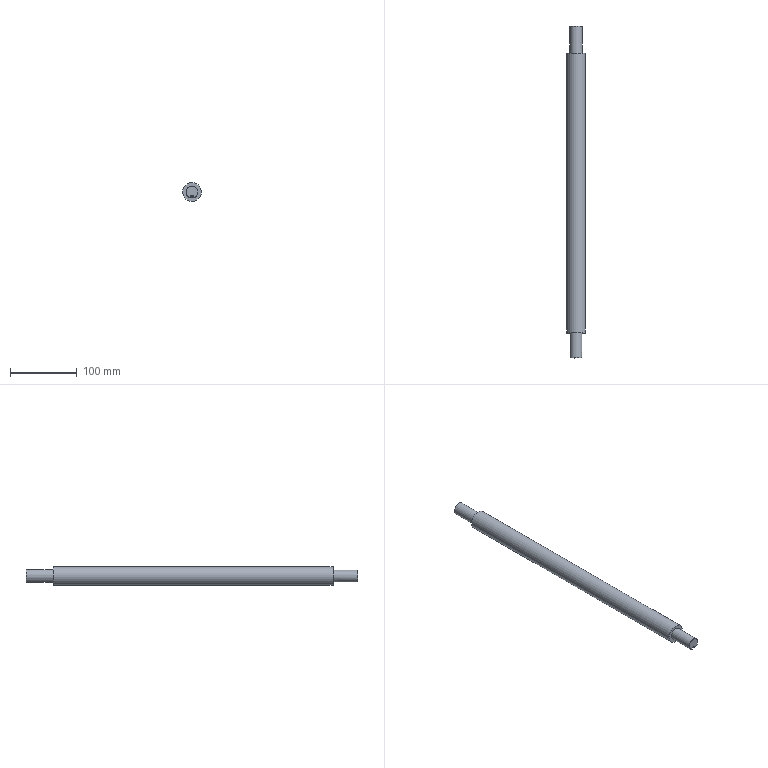Part | STEP file | SN10_002_009-03_EIXO | 1 solid | 15 faces | box 28 x 498.3 x 28 mm | volume 278975 mm3 | plane 8 | cylinder 5 | cone 2 | commonest cylinder face diameters 5 x2 18 x1 19.05 x1 28 x1
STEP:
#1=CARTESIAN_POINT('',(0.,0.,0.));
#2=DIRECTION('',(0.,0.,1.));
#3=DIRECTION('',(1.,0.,0.));
#4=AXIS2_PLACEMENT_3D('',#1,#2,#3);
#5=CARTESIAN_POINT('',(993.288,42.3,12.286));
#6=VERTEX_POINT('',#5);
#7=CARTESIAN_POINT('',(1000.,42.3,0.));
#8=DIRECTION('',(0.,-1.,0.));
#9=DIRECTION('',(1.,0.,0.));
#10=AXIS2_PLACEMENT_3D('',#7,#8,#9);
#11=CIRCLE('',#10,14.);
#12=CARTESIAN_POINT('',(1000.,-165.85,0.));
#13=DIRECTION('',(0.,-1.,0.));
#14=DIRECTION('',(-0.4794,0.,0.8776));
#15=AXIS2_PLACEMENT_3D('',#12,#13,#14);
#16=CYLINDRICAL_SURFACE('',#15,14.);
#17=CARTESIAN_POINT('',(-2.071,-208.15));
#18=DIRECTION('',(1.,0.));
#19=VECTOR('',#18,1.);
#20=LINE('',#17,#19);
#21=(GEOMETRIC_REPRESENTATION_CONTEXT(2)PARAMETRIC_REPRESENTATION_CONTEXT()REPRESENTATION_CONTEXT('',''));
#22=DEFINITIONAL_REPRESENTATION('',(#20),#21);
#23=PCURVE('',#16,#22);
#24=CARTESIAN_POINT('',(1000.,42.3,14.));
#25=DIRECTION('',(0.,-1.,0.));
#26=DIRECTION('',(0.,0.,-1.));
#27=AXIS2_PLACEMENT_3D('',#24,#25,#26);
#28=PLANE('',#27);
#29=CARTESIAN_POINT('',(14.,0.));
#30=DIRECTION('',(0.,1.));
#31=AXIS2_PLACEMENT_2D('',#29,#30);
#32=CIRCLE('',#31,14.);
#33=(GEOMETRIC_REPRESENTATION_CONTEXT(2)PARAMETRIC_REPRESENTATION_CONTEXT()REPRESENTATION_CONTEXT('',''));
#34=DEFINITIONAL_REPRESENTATION('',(#32),#33);
#35=PCURVE('',#28,#34);
#36=SURFACE_CURVE('',#11,(#23,#35),.PCURVE_S1.);
#37=EDGE_CURVE('',#6,#6,#36,.T.);
#38=ORIENTED_EDGE('',*,*,#37,.T.);
#39=CARTESIAN_POINT('',(993.288,-377.5,12.286));
#40=VERTEX_POINT('',#39);
#41=CARTESIAN_POINT('',(993.288,42.3,12.286));
#42=CARTESIAN_POINT('',(993.288,-377.5,12.286));
#43=B_SPLINE_CURVE_WITH_KNOTS('',1,(#41,#42),.UNSPECIFIED.,.F.,.F.,(2,2),(-208.15,211.65),.PIECEWISE_BEZIER_KNOTS.);
#44=CARTESIAN_POINT('',(6.283,0.));
#45=DIRECTION('',(0.,1.));
#46=VECTOR('',#45,1.);
#47=LINE('',#44,#46);
#48=(GEOMETRIC_REPRESENTATION_CONTEXT(2)PARAMETRIC_REPRESENTATION_CONTEXT()REPRESENTATION_CONTEXT('',''));
#49=DEFINITIONAL_REPRESENTATION('',(#47),#48);
#50=PCURVE('',#16,#49);
#51=CARTESIAN_POINT('',(0.,0.));
#52=DIRECTION('',(0.,1.));
#53=VECTOR('',#52,1.);
#54=LINE('',#51,#53);
#55=(GEOMETRIC_REPRESENTATION_CONTEXT(2)PARAMETRIC_REPRESENTATION_CONTEXT()REPRESENTATION_CONTEXT('',''));
#56=DEFINITIONAL_REPRESENTATION('',(#54),#55);
#57=PCURVE('',#16,#56);
#58=SEAM_CURVE('',#43,(#50,#57),.PCURVE_S1.);
#59=EDGE_CURVE('',#6,#40,#58,.T.);
#60=ORIENTED_EDGE('',*,*,#59,.T.);
#61=CARTESIAN_POINT('',(1000.,-377.5,0.));
#62=DIRECTION('',(0.,-1.,0.));
#63=DIRECTION('',(1.,0.,0.));
#64=AXIS2_PLACEMENT_3D('',#61,#62,#63);
#65=CIRCLE('',#64,14.);
#66=CARTESIAN_POINT('',(-2.071,211.65));
#67=DIRECTION('',(1.,0.));
#68=VECTOR('',#67,1.);
#69=LINE('',#66,#68);
#70=(GEOMETRIC_REPRESENTATION_CONTEXT(2)PARAMETRIC_REPRESENTATION_CONTEXT()REPRESENTATION_CONTEXT('',''));
#71=DEFINITIONAL_REPRESENTATION('',(#69),#70);
#72=PCURVE('',#16,#71);
#73=CARTESIAN_POINT('',(1000.,-377.5,9.));
#74=DIRECTION('',(0.,-1.,0.));
#75=DIRECTION('',(0.,0.,-1.));
#76=AXIS2_PLACEMENT_3D('',#73,#74,#75);
#77=PLANE('',#76);
#78=CARTESIAN_POINT('',(9.,0.));
#79=DIRECTION('',(0.,1.));
#80=AXIS2_PLACEMENT_2D('',#78,#79);
#81=CIRCLE('',#80,14.);
#82=(GEOMETRIC_REPRESENTATION_CONTEXT(2)PARAMETRIC_REPRESENTATION_CONTEXT()REPRESENTATION_CONTEXT('',''));
#83=DEFINITIONAL_REPRESENTATION('',(#81),#82);
#84=PCURVE('',#77,#83);
#85=SURFACE_CURVE('',#65,(#72,#84),.PCURVE_S1.);
#86=EDGE_CURVE('',#40,#40,#85,.T.);
#87=ORIENTED_EDGE('',*,*,#86,.F.);
#88=ORIENTED_EDGE('',*,*,#59,.F.);
#89=EDGE_LOOP('',(#38,#60,#87,#88));
#90=FACE_BOUND('',#89,.T.);
#91=ADVANCED_FACE('',(#90),#16,.T.);
#92=ORIENTED_EDGE('',*,*,#37,.F.);
#93=EDGE_LOOP('',(#92));
#94=FACE_BOUND('',#93,.T.);
#95=CARTESIAN_POINT('',(995.433,42.3,8.359));
#96=VERTEX_POINT('',#95);
#97=CARTESIAN_POINT('',(1000.,42.3,0.));
#98=DIRECTION('',(0.,-1.,0.));
#99=DIRECTION('',(1.,0.,0.));
#100=AXIS2_PLACEMENT_3D('',#97,#98,#99);
#101=CIRCLE('',#100,9.525);
#102=CARTESIAN_POINT('',(14.,0.));
#103=DIRECTION('',(0.,1.));
#104=AXIS2_PLACEMENT_2D('',#102,#103);
#105=CIRCLE('',#104,9.525);
#106=(GEOMETRIC_REPRESENTATION_CONTEXT(2)PARAMETRIC_REPRESENTATION_CONTEXT()REPRESENTATION_CONTEXT('',''));
#107=DEFINITIONAL_REPRESENTATION('',(#105),#106);
#108=PCURVE('',#28,#107);
#109=CARTESIAN_POINT('',(1000.,-165.85,0.));
#110=DIRECTION('',(0.,-1.,0.));
#111=DIRECTION('',(-0.4794,0.,0.8776));
#112=AXIS2_PLACEMENT_3D('',#109,#110,#111);
#113=CYLINDRICAL_SURFACE('',#112,9.525);
#114=CARTESIAN_POINT('',(-2.071,-208.15));
#115=DIRECTION('',(1.,0.));
#116=VECTOR('',#115,1.);
#117=LINE('',#114,#116);
#118=(GEOMETRIC_REPRESENTATION_CONTEXT(2)PARAMETRIC_REPRESENTATION_CONTEXT()REPRESENTATION_CONTEXT('',''));
#119=DEFINITIONAL_REPRESENTATION('',(#117),#118);
#120=PCURVE('',#113,#119);
#121=SURFACE_CURVE('',#101,(#108,#120),.PCURVE_S1.);
#122=EDGE_CURVE('',#96,#96,#121,.T.);
#123=ORIENTED_EDGE('',*,*,#122,.T.);
#124=EDGE_LOOP('',(#123));
#125=FACE_BOUND('',#124,.T.);
#126=ADVANCED_FACE('',(#94,#125),#28,.F.);
#127=ORIENTED_EDGE('',*,*,#86,.T.);
#128=EDGE_LOOP('',(#127));
#129=FACE_BOUND('',#128,.T.);
#130=CARTESIAN_POINT('',(995.685,-377.5,7.898));
#131=VERTEX_POINT('',#130);
#132=CARTESIAN_POINT('',(1000.,-377.5,0.));
#133=DIRECTION('',(0.,-1.,0.));
#134=DIRECTION('',(1.,0.,0.));
#135=AXIS2_PLACEMENT_3D('',#132,#133,#134);
#136=CIRCLE('',#135,9.);
#137=CARTESIAN_POINT('',(9.,0.));
#138=DIRECTION('',(0.,1.));
#139=AXIS2_PLACEMENT_2D('',#137,#138);
#140=CIRCLE('',#139,9.);
#141=(GEOMETRIC_REPRESENTATION_CONTEXT(2)PARAMETRIC_REPRESENTATION_CONTEXT()REPRESENTATION_CONTEXT('',''));
#142=DEFINITIONAL_REPRESENTATION('',(#140),#141);
#143=PCURVE('',#77,#142);
#144=CARTESIAN_POINT('',(1000.,-165.85,0.));
#145=DIRECTION('',(0.,-1.,0.));
#146=DIRECTION('',(-0.4794,0.,0.8776));
#147=AXIS2_PLACEMENT_3D('',#144,#145,#146);
#148=CYLINDRICAL_SURFACE('',#147,9.);
#149=CARTESIAN_POINT('',(-2.071,211.65));
#150=DIRECTION('',(1.,0.));
#151=VECTOR('',#150,1.);
#152=LINE('',#149,#151);
#153=(GEOMETRIC_REPRESENTATION_CONTEXT(2)PARAMETRIC_REPRESENTATION_CONTEXT()REPRESENTATION_CONTEXT('',''));
#154=DEFINITIONAL_REPRESENTATION('',(#152),#153);
#155=PCURVE('',#148,#154);
#156=SURFACE_CURVE('',#136,(#143,#155),.PCURVE_S1.);
#157=EDGE_CURVE('',#131,#131,#156,.T.);
#158=ORIENTED_EDGE('',*,*,#157,.F.);
#159=EDGE_LOOP('',(#158));
#160=FACE_BOUND('',#159,.T.);
#161=ADVANCED_FACE('',(#129,#160),#77,.T.);
#162=CARTESIAN_POINT('',(995.685,-414.5,7.898));
#163=VERTEX_POINT('',#162);
#164=CARTESIAN_POINT('',(997.,-414.5,-8.485));
#165=VERTEX_POINT('',#164);
#166=CARTESIAN_POINT('',(1000.,-414.5,0.));
#167=DIRECTION('',(0.,-1.,0.));
#168=DIRECTION('',(1.,0.,0.));
#169=AXIS2_PLACEMENT_3D('',#166,#167,#168);
#170=CIRCLE('',#169,9.);
#171=CARTESIAN_POINT('',(-2.071,248.65));
#172=DIRECTION('',(1.,0.));
#173=VECTOR('',#172,1.);
#174=LINE('',#171,#173);
#175=(GEOMETRIC_REPRESENTATION_CONTEXT(2)PARAMETRIC_REPRESENTATION_CONTEXT()REPRESENTATION_CONTEXT('',''));
#176=DEFINITIONAL_REPRESENTATION('',(#174),#175);
#177=PCURVE('',#148,#176);
#178=CARTESIAN_POINT('',(1000.,-422.5,0.));
#179=DIRECTION('',(0.,1.,0.));
#180=DIRECTION('',(0.3128,0.,-0.9498));
#181=AXIS2_PLACEMENT_3D('',#178,#179,#180);
#182=CONICAL_SURFACE('',#181,1.,0.7854);
#183=CARTESIAN_POINT('',(5.031,8.));
#184=DIRECTION('',(-1.,0.));
#185=VECTOR('',#184,1.);
#186=LINE('',#183,#185);
#187=(GEOMETRIC_REPRESENTATION_CONTEXT(2)PARAMETRIC_REPRESENTATION_CONTEXT()REPRESENTATION_CONTEXT('',''));
#188=DEFINITIONAL_REPRESENTATION('',(#186),#187);
#189=PCURVE('',#182,#188);
#190=SURFACE_CURVE('',#170,(#177,#189),.PCURVE_S1.);
#191=EDGE_CURVE('',#163,#165,#190,.T.);
#192=ORIENTED_EDGE('',*,*,#191,.F.);
#193=CARTESIAN_POINT('',(995.685,-377.5,7.898));
#194=CARTESIAN_POINT('',(995.685,-414.5,7.898));
#195=B_SPLINE_CURVE_WITH_KNOTS('',1,(#193,#194),.UNSPECIFIED.,.F.,.F.,(2,2),(211.65,248.65),.PIECEWISE_BEZIER_KNOTS.);
#196=CARTESIAN_POINT('',(0.,0.));
#197=DIRECTION('',(0.,1.));
#198=VECTOR('',#197,1.);
#199=LINE('',#196,#198);
#200=(GEOMETRIC_REPRESENTATION_CONTEXT(2)PARAMETRIC_REPRESENTATION_CONTEXT()REPRESENTATION_CONTEXT('',''));
#201=DEFINITIONAL_REPRESENTATION('',(#199),#200);
#202=PCURVE('',#148,#201);
#203=CARTESIAN_POINT('',(6.283,0.));
#204=DIRECTION('',(0.,1.));
#205=VECTOR('',#204,1.);
#206=LINE('',#203,#205);
#207=(GEOMETRIC_REPRESENTATION_CONTEXT(2)PARAMETRIC_REPRESENTATION_CONTEXT()REPRESENTATION_CONTEXT('',''));
#208=DEFINITIONAL_REPRESENTATION('',(#206),#207);
#209=PCURVE('',#148,#208);
#210=SEAM_CURVE('',#195,(#202,#209),.PCURVE_S1.);
#211=EDGE_CURVE('',#131,#163,#210,.T.);
#212=ORIENTED_EDGE('',*,*,#211,.F.);
#213=ORIENTED_EDGE('',*,*,#157,.T.);
#214=ORIENTED_EDGE('',*,*,#211,.T.);
#215=CARTESIAN_POINT('',(1003.,-414.5,-8.485));
#216=VERTEX_POINT('',#215);
#217=CARTESIAN_POINT('',(1000.,-414.5,0.));
#218=DIRECTION('',(0.,-1.,0.));
#219=DIRECTION('',(1.,0.,0.));
#220=AXIS2_PLACEMENT_3D('',#217,#218,#219);
#221=CIRCLE('',#220,9.);
#222=CARTESIAN_POINT('',(-2.071,248.65));
#223=DIRECTION('',(1.,0.));
#224=VECTOR('',#223,1.);
#225=LINE('',#222,#224);
#226=(GEOMETRIC_REPRESENTATION_CONTEXT(2)PARAMETRIC_REPRESENTATION_CONTEXT()REPRESENTATION_CONTEXT('',''));
#227=DEFINITIONAL_REPRESENTATION('',(#225),#226);
#228=PCURVE('',#148,#227);
#229=CARTESIAN_POINT('',(11.314,8.));
#230=DIRECTION('',(-1.,0.));
#231=VECTOR('',#230,1.);
#232=LINE('',#229,#231);
#233=(GEOMETRIC_REPRESENTATION_CONTEXT(2)PARAMETRIC_REPRESENTATION_CONTEXT()REPRESENTATION_CONTEXT('',''));
#234=DEFINITIONAL_REPRESENTATION('',(#232),#233);
#235=PCURVE('',#182,#234);
#236=SURFACE_CURVE('',#221,(#228,#235),.PCURVE_S1.);
#237=EDGE_CURVE('',#216,#163,#236,.T.);
#238=ORIENTED_EDGE('',*,*,#237,.F.);
#239=CARTESIAN_POINT('',(1003.,-382.5,-8.485));
#240=VERTEX_POINT('',#239);
#241=CARTESIAN_POINT('',(1003.,-382.5,-8.485));
#242=DIRECTION('',(0.,-1.,0.));
#243=VECTOR('',#242,1.);
#244=LINE('',#241,#243);
#245=CARTESIAN_POINT('',(2.981,216.65));
#246=DIRECTION('',(0.,1.));
#247=VECTOR('',#246,1.);
#248=LINE('',#245,#247);
#249=(GEOMETRIC_REPRESENTATION_CONTEXT(2)PARAMETRIC_REPRESENTATION_CONTEXT()REPRESENTATION_CONTEXT('',''));
#250=DEFINITIONAL_REPRESENTATION('',(#248),#249);
#251=PCURVE('',#148,#250);
#252=CARTESIAN_POINT('',(1003.,-415.,-11.3));
#253=DIRECTION('',(-1.,0.,0.));
#254=DIRECTION('',(0.,0.,1.));
#255=AXIS2_PLACEMENT_3D('',#252,#253,#254);
#256=PLANE('',#255);
#257=CARTESIAN_POINT('',(2.815,32.5));
#258=DIRECTION('',(0.,-1.));
#259=VECTOR('',#258,1.);
#260=LINE('',#257,#259);
#261=(GEOMETRIC_REPRESENTATION_CONTEXT(2)PARAMETRIC_REPRESENTATION_CONTEXT()REPRESENTATION_CONTEXT('',''));
#262=DEFINITIONAL_REPRESENTATION('',(#260),#261);
#263=PCURVE('',#256,#262);
#264=SURFACE_CURVE('',#244,(#251,#263),.PCURVE_S1.);
#265=EDGE_CURVE('',#240,#216,#264,.T.);
#266=ORIENTED_EDGE('',*,*,#265,.F.);
#267=CARTESIAN_POINT('',(1000.5,-380.,-8.986));
#268=VERTEX_POINT('',#267);
#269=CARTESIAN_POINT('',(1003.,-382.5,-8.485));
#270=CARTESIAN_POINT('',(1003.,-382.184,-8.485));
#271=CARTESIAN_POINT('',(1002.936,-381.849,-8.509));
#272=CARTESIAN_POINT('',(1002.682,-381.235,-8.592));
#273=CARTESIAN_POINT('',(1002.49,-380.956,-8.652));
#274=CARTESIAN_POINT('',(1002.05,-380.514,-8.766));
#275=CARTESIAN_POINT('',(1001.77,-380.321,-8.83));
#276=CARTESIAN_POINT('',(1001.154,-380.064,-8.931));
#277=CARTESIAN_POINT('',(1000.818,-380.,-8.968));
#278=CARTESIAN_POINT('',(1000.5,-380.,-8.986));
#279=B_SPLINE_CURVE_WITH_KNOTS('',3,(#269,#270,#271,#272,#273,#274,#275,#276,#277,#278),.UNSPECIFIED.,.F.,.F.,(4,2,2,2,4),(-0.7583,-0.6635,-0.5687,-0.4733,-0.3778),.UNSPECIFIED.);
#280=CARTESIAN_POINT('',(2.981,216.65));
#281=CARTESIAN_POINT('',(2.981,216.592));
#282=CARTESIAN_POINT('',(2.981,216.476));
#283=CARTESIAN_POINT('',(2.979,216.299));
#284=CARTESIAN_POINT('',(2.975,216.121));
#285=CARTESIAN_POINT('',(2.97,215.945));
#286=CARTESIAN_POINT('',(2.963,215.772));
#287=CARTESIAN_POINT('',(2.955,215.604));
#288=CARTESIAN_POINT('',(2.945,215.442));
#289=CARTESIAN_POINT('',(2.934,215.288));
#290=CARTESIAN_POINT('',(2.923,215.142));
#291=CARTESIAN_POINT('',(2.91,215.005));
#292=CARTESIAN_POINT('',(2.896,214.88));
#293=CARTESIAN_POINT('',(2.882,214.763));
#294=CARTESIAN_POINT('',(2.866,214.652));
#295=CARTESIAN_POINT('',(2.85,214.55));
#296=CARTESIAN_POINT('',(2.832,214.458));
#297=CARTESIAN_POINT('',(2.814,214.376));
#298=CARTESIAN_POINT('',(2.795,214.306));
#299=CARTESIAN_POINT('',(2.776,214.249));
#300=CARTESIAN_POINT('',(2.756,214.205));
#301=CARTESIAN_POINT('',(2.736,214.173));
#302=CARTESIAN_POINT('',(2.717,214.154));
#303=CARTESIAN_POINT('',(2.704,214.15));
#304=CARTESIAN_POINT('',(2.697,214.15));
#305=B_SPLINE_CURVE_WITH_KNOTS('',3,(#280,#281,#282,#283,#284,#285,#286,#287,#288,#289,#290,#291,#292,#293,#294,#295,#296,#297,#298,#299,#300,#301,#302,#303,#304),.UNSPECIFIED.,.F.,.F.,(4,1,1,1,1,1,1,1,1,1,1,1,1,1,1,1,1,1,1,1,1,1,4),(-0.7583,-0.741,-0.7238,-0.7065,-0.6892,-0.6719,-0.6546,-0.6373,-0.62,-0.6027,-0.5854,-0.5681,-0.5508,-0.5335,-0.5162,-0.4989,-0.4816,-0.4643,-0.447,-0.4297,-0.4124,-0.3951,-0.3778),.QUASI_UNIFORM_KNOTS.);
#306=(GEOMETRIC_REPRESENTATION_CONTEXT(2)PARAMETRIC_REPRESENTATION_CONTEXT()REPRESENTATION_CONTEXT('',''));
#307=DEFINITIONAL_REPRESENTATION('',(#305),#306);
#308=PCURVE('',#148,#307);
#309=CARTESIAN_POINT('',(1000.5,-382.5,-7.15));
#310=DIRECTION('',(0.,0.,1.));
#311=DIRECTION('',(1.,0.,0.));
#312=AXIS2_PLACEMENT_3D('',#309,#310,#311);
#313=CYLINDRICAL_SURFACE('',#312,2.5);
#314=CARTESIAN_POINT('',(0.,-1.335));
#315=CARTESIAN_POINT('',(0.02306,-1.335));
#316=CARTESIAN_POINT('',(0.0697,-1.337));
#317=CARTESIAN_POINT('',(0.1409,-1.344));
#318=CARTESIAN_POINT('',(0.2129,-1.355));
#319=CARTESIAN_POINT('',(0.2855,-1.37));
#320=CARTESIAN_POINT('',(0.3584,-1.389));
#321=CARTESIAN_POINT('',(0.4312,-1.412));
#322=CARTESIAN_POINT('',(0.5038,-1.438));
#323=CARTESIAN_POINT('',(0.5759,-1.467));
#324=CARTESIAN_POINT('',(0.6472,-1.497));
#325=CARTESIAN_POINT('',(0.7176,-1.529));
#326=CARTESIAN_POINT('',(0.7861,-1.56));
#327=CARTESIAN_POINT('',(0.8547,-1.592));
#328=CARTESIAN_POINT('',(0.925,-1.624));
#329=CARTESIAN_POINT('',(0.9963,-1.656));
#330=CARTESIAN_POINT('',(1.068,-1.687));
#331=CARTESIAN_POINT('',(1.141,-1.717));
#332=CARTESIAN_POINT('',(1.213,-1.745));
#333=CARTESIAN_POINT('',(1.286,-1.77));
#334=CARTESIAN_POINT('',(1.358,-1.791));
#335=CARTESIAN_POINT('',(1.43,-1.81));
#336=CARTESIAN_POINT('',(1.501,-1.825));
#337=CARTESIAN_POINT('',(1.548,-1.833));
#338=CARTESIAN_POINT('',(1.571,-1.836));
#339=B_SPLINE_CURVE_WITH_KNOTS('',3,(#314,#315,#316,#317,#318,#319,#320,#321,#322,#323,#324,#325,#326,#327,#328,#329,#330,#331,#332,#333,#334,#335,#336,#337,#338),.UNSPECIFIED.,.F.,.F.,(4,1,1,1,1,1,1,1,1,1,1,1,1,1,1,1,1,1,1,1,1,1,4),(-0.7583,-0.741,-0.7238,-0.7065,-0.6892,-0.6719,-0.6546,-0.6373,-0.62,-0.6027,-0.5854,-0.5681,-0.5508,-0.5335,-0.5162,-0.4989,-0.4816,-0.4643,-0.447,-0.4297,-0.4124,-0.3951,-0.3778),.QUASI_UNIFORM_KNOTS.);
#340=(GEOMETRIC_REPRESENTATION_CONTEXT(2)PARAMETRIC_REPRESENTATION_CONTEXT()REPRESENTATION_CONTEXT('',''));
#341=DEFINITIONAL_REPRESENTATION('',(#339),#340);
#342=PCURVE('',#313,#341);
#343=SURFACE_CURVE('',#279,(#308,#342),.PCURVE_S1.);
#344=EDGE_CURVE('',#240,#268,#343,.T.);
#345=ORIENTED_EDGE('',*,*,#344,.T.);
#346=CARTESIAN_POINT('',(999.5,-380.,-8.986));
#347=VERTEX_POINT('',#346);
#348=CARTESIAN_POINT('',(1000.,-380.,0.));
#349=DIRECTION('',(0.,-1.,0.));
#350=DIRECTION('',(1.,0.,0.));
#351=AXIS2_PLACEMENT_3D('',#348,#349,#350);
#352=CIRCLE('',#351,9.);
#353=CARTESIAN_POINT('',(-2.071,214.15));
#354=DIRECTION('',(1.,0.));
#355=VECTOR('',#354,1.);
#356=LINE('',#353,#355);
#357=(GEOMETRIC_REPRESENTATION_CONTEXT(2)PARAMETRIC_REPRESENTATION_CONTEXT()REPRESENTATION_CONTEXT('',''));
#358=DEFINITIONAL_REPRESENTATION('',(#356),#357);
#359=PCURVE('',#148,#358);
#360=CARTESIAN_POINT('',(0.,-380.,0.));
#361=DIRECTION('',(0.,-1.,0.));
#362=DIRECTION('',(0.,0.,-1.));
#363=AXIS2_PLACEMENT_3D('',#360,#361,#362);
#364=PLANE('',#363);
#365=CARTESIAN_POINT('',(0.,1000.));
#366=DIRECTION('',(0.,1.));
#367=AXIS2_PLACEMENT_2D('',#365,#366);
#368=CIRCLE('',#367,9.);
#369=(GEOMETRIC_REPRESENTATION_CONTEXT(2)PARAMETRIC_REPRESENTATION_CONTEXT()REPRESENTATION_CONTEXT('',''));
#370=DEFINITIONAL_REPRESENTATION('',(#368),#369);
#371=PCURVE('',#364,#370);
#372=SURFACE_CURVE('',#352,(#359,#371),.PCURVE_S1.);
#373=EDGE_CURVE('',#347,#268,#372,.T.);
#374=ORIENTED_EDGE('',*,*,#373,.F.);
#375=CARTESIAN_POINT('',(997.,-382.5,-8.485));
#376=VERTEX_POINT('',#375);
#377=CARTESIAN_POINT('',(997.,-382.5,-8.485));
#378=CARTESIAN_POINT('',(997.,-382.184,-8.485));
#379=CARTESIAN_POINT('',(997.064,-381.849,-8.509));
#380=CARTESIAN_POINT('',(997.318,-381.235,-8.592));
#381=CARTESIAN_POINT('',(997.51,-380.956,-8.652));
#382=CARTESIAN_POINT('',(997.95,-380.514,-8.766));
#383=CARTESIAN_POINT('',(998.23,-380.321,-8.83));
#384=CARTESIAN_POINT('',(998.846,-380.064,-8.931));
#385=CARTESIAN_POINT('',(999.182,-380.,-8.968));
#386=CARTESIAN_POINT('',(999.5,-380.,-8.986));
#387=B_SPLINE_CURVE_WITH_KNOTS('',3,(#377,#378,#379,#380,#381,#382,#383,#384,#385,#386),.UNSPECIFIED.,.F.,.F.,(4,2,2,2,4),(-0.7583,-0.6635,-0.5687,-0.4733,-0.3778),.UNSPECIFIED.);
#388=CARTESIAN_POINT('',(2.302,216.65));
#389=CARTESIAN_POINT('',(2.302,216.592));
#390=CARTESIAN_POINT('',(2.302,216.476));
#391=CARTESIAN_POINT('',(2.305,216.299));
#392=CARTESIAN_POINT('',(2.308,216.121));
#393=CARTESIAN_POINT('',(2.313,215.945));
#394=CARTESIAN_POINT('',(2.32,215.772));
#395=CARTESIAN_POINT('',(2.328,215.604));
#396=CARTESIAN_POINT('',(2.338,215.442));
#397=CARTESIAN_POINT('',(2.349,215.288));
#398=CARTESIAN_POINT('',(2.361,215.142));
#399=CARTESIAN_POINT('',(2.373,215.005));
#400=CARTESIAN_POINT('',(2.387,214.88));
#401=CARTESIAN_POINT('',(2.401,214.763));
#402=CARTESIAN_POINT('',(2.417,214.652));
#403=CARTESIAN_POINT('',(2.434,214.55));
#404=CARTESIAN_POINT('',(2.451,214.458));
#405=CARTESIAN_POINT('',(2.469,214.376));
#406=CARTESIAN_POINT('',(2.488,214.306));
#407=CARTESIAN_POINT('',(2.508,214.249));
#408=CARTESIAN_POINT('',(2.527,214.205));
#409=CARTESIAN_POINT('',(2.547,214.173));
#410=CARTESIAN_POINT('',(2.567,214.154));
#411=CARTESIAN_POINT('',(2.58,214.15));
#412=CARTESIAN_POINT('',(2.586,214.15));
#413=B_SPLINE_CURVE_WITH_KNOTS('',3,(#388,#389,#390,#391,#392,#393,#394,#395,#396,#397,#398,#399,#400,#401,#402,#403,#404,#405,#406,#407,#408,#409,#410,#411,#412),.UNSPECIFIED.,.F.,.F.,(4,1,1,1,1,1,1,1,1,1,1,1,1,1,1,1,1,1,1,1,1,1,4),(-0.7583,-0.741,-0.7238,-0.7065,-0.6892,-0.6719,-0.6546,-0.6373,-0.62,-0.6027,-0.5854,-0.5681,-0.5508,-0.5335,-0.5162,-0.4989,-0.4816,-0.4643,-0.447,-0.4297,-0.4124,-0.3951,-0.3778),.QUASI_UNIFORM_KNOTS.);
#414=(GEOMETRIC_REPRESENTATION_CONTEXT(2)PARAMETRIC_REPRESENTATION_CONTEXT()REPRESENTATION_CONTEXT('',''));
#415=DEFINITIONAL_REPRESENTATION('',(#413),#414);
#416=PCURVE('',#148,#415);
#417=CARTESIAN_POINT('',(999.5,-382.5,-7.15));
#418=DIRECTION('',(0.,0.,-1.));
#419=DIRECTION('',(-1.,0.,0.));
#420=AXIS2_PLACEMENT_3D('',#417,#418,#419);
#421=CYLINDRICAL_SURFACE('',#420,2.5);
#422=CARTESIAN_POINT('',(0.,1.335));
#423=CARTESIAN_POINT('',(0.02306,1.335));
#424=CARTESIAN_POINT('',(0.0697,1.337));
#425=CARTESIAN_POINT('',(0.1409,1.344));
#426=CARTESIAN_POINT('',(0.2129,1.355));
#427=CARTESIAN_POINT('',(0.2855,1.37));
#428=CARTESIAN_POINT('',(0.3584,1.389));
#429=CARTESIAN_POINT('',(0.4312,1.412));
#430=CARTESIAN_POINT('',(0.5038,1.438));
#431=CARTESIAN_POINT('',(0.5759,1.467));
#432=CARTESIAN_POINT('',(0.6472,1.497));
#433=CARTESIAN_POINT('',(0.7176,1.529));
#434=CARTESIAN_POINT('',(0.7861,1.56));
#435=CARTESIAN_POINT('',(0.8547,1.592));
#436=CARTESIAN_POINT('',(0.925,1.624));
#437=CARTESIAN_POINT('',(0.9963,1.656));
#438=CARTESIAN_POINT('',(1.068,1.687));
#439=CARTESIAN_POINT('',(1.141,1.717));
#440=CARTESIAN_POINT('',(1.213,1.745));
#441=CARTESIAN_POINT('',(1.286,1.77));
#442=CARTESIAN_POINT('',(1.358,1.791));
#443=CARTESIAN_POINT('',(1.43,1.81));
#444=CARTESIAN_POINT('',(1.501,1.825));
#445=CARTESIAN_POINT('',(1.548,1.833));
#446=CARTESIAN_POINT('',(1.571,1.836));
#447=B_SPLINE_CURVE_WITH_KNOTS('',3,(#422,#423,#424,#425,#426,#427,#428,#429,#430,#431,#432,#433,#434,#435,#436,#437,#438,#439,#440,#441,#442,#443,#444,#445,#446),.UNSPECIFIED.,.F.,.F.,(4,1,1,1,1,1,1,1,1,1,1,1,1,1,1,1,1,1,1,1,1,1,4),(-0.7583,-0.741,-0.7238,-0.7065,-0.6892,-0.6719,-0.6546,-0.6373,-0.62,-0.6027,-0.5854,-0.5681,-0.5508,-0.5335,-0.5162,-0.4989,-0.4816,-0.4643,-0.447,-0.4297,-0.4124,-0.3951,-0.3778),.QUASI_UNIFORM_KNOTS.);
#448=(GEOMETRIC_REPRESENTATION_CONTEXT(2)PARAMETRIC_REPRESENTATION_CONTEXT()REPRESENTATION_CONTEXT('',''));
#449=DEFINITIONAL_REPRESENTATION('',(#447),#448);
#450=PCURVE('',#421,#449);
#451=SURFACE_CURVE('',#387,(#416,#450),.PCURVE_S1.);
#452=EDGE_CURVE('',#376,#347,#451,.T.);
#453=ORIENTED_EDGE('',*,*,#452,.F.);
#454=CARTESIAN_POINT('',(997.,-414.5,-8.485));
#455=DIRECTION('',(0.,1.,0.));
#456=VECTOR('',#455,1.);
#457=LINE('',#454,#456);
#458=CARTESIAN_POINT('',(2.302,248.65));
#459=DIRECTION('',(0.,-1.));
#460=VECTOR('',#459,1.);
#461=LINE('',#458,#460);
#462=(GEOMETRIC_REPRESENTATION_CONTEXT(2)PARAMETRIC_REPRESENTATION_CONTEXT()REPRESENTATION_CONTEXT('',''));
#463=DEFINITIONAL_REPRESENTATION('',(#461),#462);
#464=PCURVE('',#148,#463);
#465=CARTESIAN_POINT('',(997.,-415.,-5.3));
#466=DIRECTION('',(1.,0.,0.));
#467=DIRECTION('',(0.,0.,-1.));
#468=AXIS2_PLACEMENT_3D('',#465,#466,#467);
#469=PLANE('',#468);
#470=CARTESIAN_POINT('',(3.185,0.5));
#471=DIRECTION('',(0.,1.));
#472=VECTOR('',#471,1.);
#473=LINE('',#470,#472);
#474=(GEOMETRIC_REPRESENTATION_CONTEXT(2)PARAMETRIC_REPRESENTATION_CONTEXT()REPRESENTATION_CONTEXT('',''));
#475=DEFINITIONAL_REPRESENTATION('',(#473),#474);
#476=PCURVE('',#469,#475);
#477=SURFACE_CURVE('',#457,(#464,#476),.PCURVE_S1.);
#478=EDGE_CURVE('',#165,#376,#477,.T.);
#479=ORIENTED_EDGE('',*,*,#478,.F.);
#480=EDGE_LOOP('',(#192,#212,#213,#214,#238,#266,#345,#374,#453,#479));
#481=FACE_BOUND('',#480,.T.);
#482=ADVANCED_FACE('',(#481),#148,.T.);
#483=ORIENTED_EDGE('',*,*,#237,.T.);
#484=ORIENTED_EDGE('',*,*,#191,.T.);
#485=CARTESIAN_POINT('',(997.,-415.,-7.953));
#486=VERTEX_POINT('',#485);
#487=CARTESIAN_POINT('',(997.,-416.,-6.874));
#488=CARTESIAN_POINT('',(997.,-411.137,-12.18));
#489=CARTESIAN_POINT('',(997.,-381.5,-41.893));
#490=(BOUNDED_CURVE()B_SPLINE_CURVE(2,(#487,#488,#489),.UNSPECIFIED.,.F.,.F.)B_SPLINE_CURVE_WITH_KNOTS((3,3),(0.,4.916),.PIECEWISE_BEZIER_KNOTS.)CURVE()GEOMETRIC_REPRESENTATION_ITEM()RATIONAL_B_SPLINE_CURVE((1.,1.415,1.))REPRESENTATION_ITEM(''));
#491=CARTESIAN_POINT('',(0.6789,7.5));
#492=CARTESIAN_POINT('',(0.658,8.));
#493=B_SPLINE_CURVE_WITH_KNOTS('',1,(#491,#492),.UNSPECIFIED.,.F.,.F.,(2,2),(0.3408,0.4999),.PIECEWISE_BEZIER_KNOTS.);
#494=(GEOMETRIC_REPRESENTATION_CONTEXT(2)PARAMETRIC_REPRESENTATION_CONTEXT()REPRESENTATION_CONTEXT('',''));
#495=DEFINITIONAL_REPRESENTATION('',(#493),#494);
#496=PCURVE('',#182,#495);
#497=CARTESIAN_POINT('',(1.574,-1.));
#498=CARTESIAN_POINT('',(6.88,3.863));
#499=CARTESIAN_POINT('',(36.593,33.5));
#500=(BOUNDED_CURVE()B_SPLINE_CURVE(2,(#497,#498,#499),.UNSPECIFIED.,.F.,.F.)B_SPLINE_CURVE_WITH_KNOTS((3,3),(0.,4.916),.PIECEWISE_BEZIER_KNOTS.)CURVE()GEOMETRIC_REPRESENTATION_ITEM()RATIONAL_B_SPLINE_CURVE((1.,1.415,1.))REPRESENTATION_ITEM(''));
#501=(GEOMETRIC_REPRESENTATION_CONTEXT(2)PARAMETRIC_REPRESENTATION_CONTEXT()REPRESENTATION_CONTEXT('',''));
#502=DEFINITIONAL_REPRESENTATION('',(#500),#501);
#503=PCURVE('',#469,#502);
#504=SURFACE_CURVE('',#490,(#496,#503),.PCURVE_S1.);
#505=EDGE_CURVE('',#486,#165,#504,.T.);
#506=ORIENTED_EDGE('',*,*,#505,.F.);
#507=CARTESIAN_POINT('',(1003.,-415.,-7.953));
#508=VERTEX_POINT('',#507);
#509=CARTESIAN_POINT('',(1000.,-415.,0.));
#510=DIRECTION('',(0.,-1.,0.));
#511=DIRECTION('',(1.,0.,0.));
#512=AXIS2_PLACEMENT_3D('',#509,#510,#511);
#513=CIRCLE('',#512,8.5);
#514=CARTESIAN_POINT('',(11.314,7.5));
#515=DIRECTION('',(-1.,0.));
#516=VECTOR('',#515,1.);
#517=LINE('',#514,#516);
#518=(GEOMETRIC_REPRESENTATION_CONTEXT(2)PARAMETRIC_REPRESENTATION_CONTEXT()REPRESENTATION_CONTEXT('',''));
#519=DEFINITIONAL_REPRESENTATION('',(#517),#518);
#520=PCURVE('',#182,#519);
#521=CARTESIAN_POINT('',(1000.,-415.,0.));
#522=DIRECTION('',(0.,-1.,0.));
#523=DIRECTION('',(0.,0.,-1.));
#524=AXIS2_PLACEMENT_3D('',#521,#522,#523);
#525=PLANE('',#524);
#526=CARTESIAN_POINT('',(0.,0.));
#527=DIRECTION('',(0.,1.));
#528=AXIS2_PLACEMENT_2D('',#526,#527);
#529=CIRCLE('',#528,8.5);
#530=(GEOMETRIC_REPRESENTATION_CONTEXT(2)PARAMETRIC_REPRESENTATION_CONTEXT()REPRESENTATION_CONTEXT('',''));
#531=DEFINITIONAL_REPRESENTATION('',(#529),#530);
#532=PCURVE('',#525,#531);
#533=SURFACE_CURVE('',#513,(#520,#532),.PCURVE_S1.);
#534=EDGE_CURVE('',#508,#486,#533,.T.);
#535=ORIENTED_EDGE('',*,*,#534,.F.);
#536=CARTESIAN_POINT('',(1003.,-416.,-6.874));
#537=CARTESIAN_POINT('',(1003.,-411.137,-12.18));
#538=CARTESIAN_POINT('',(1003.,-381.5,-41.893));
#539=(BOUNDED_CURVE()B_SPLINE_CURVE(2,(#536,#537,#538),.UNSPECIFIED.,.F.,.F.)B_SPLINE_CURVE_WITH_KNOTS((3,3),(0.,4.916),.PIECEWISE_BEZIER_KNOTS.)CURVE()GEOMETRIC_REPRESENTATION_ITEM()RATIONAL_B_SPLINE_CURVE((1.,1.415,1.))REPRESENTATION_ITEM(''));
#540=CARTESIAN_POINT('',(6.241,7.5));
#541=CARTESIAN_POINT('',(6.261,8.));
#542=B_SPLINE_CURVE_WITH_KNOTS('',1,(#540,#541),.UNSPECIFIED.,.F.,.F.,(2,2),(0.3408,0.4999),.PIECEWISE_BEZIER_KNOTS.);
#543=(GEOMETRIC_REPRESENTATION_CONTEXT(2)PARAMETRIC_REPRESENTATION_CONTEXT()REPRESENTATION_CONTEXT('',''));
#544=DEFINITIONAL_REPRESENTATION('',(#542),#543);
#545=PCURVE('',#182,#544);
#546=CARTESIAN_POINT('',(4.426,-1.));
#547=CARTESIAN_POINT('',(-0.8798,3.863));
#548=CARTESIAN_POINT('',(-30.593,33.5));
#549=(BOUNDED_CURVE()B_SPLINE_CURVE(2,(#546,#547,#548),.UNSPECIFIED.,.F.,.F.)B_SPLINE_CURVE_WITH_KNOTS((3,3),(0.,4.916),.PIECEWISE_BEZIER_KNOTS.)CURVE()GEOMETRIC_REPRESENTATION_ITEM()RATIONAL_B_SPLINE_CURVE((1.,1.415,1.))REPRESENTATION_ITEM(''));
#550=(GEOMETRIC_REPRESENTATION_CONTEXT(2)PARAMETRIC_REPRESENTATION_CONTEXT()REPRESENTATION_CONTEXT('',''));
#551=DEFINITIONAL_REPRESENTATION('',(#549),#550);
#552=PCURVE('',#256,#551);
#553=SURFACE_CURVE('',#539,(#545,#552),.PCURVE_S1.);
#554=EDGE_CURVE('',#508,#216,#553,.T.);
#555=ORIENTED_EDGE('',*,*,#554,.T.);
#556=EDGE_LOOP('',(#483,#484,#506,#535,#555));
#557=FACE_BOUND('',#556,.T.);
#558=ADVANCED_FACE('',(#557),#182,.T.);
#559=CARTESIAN_POINT('',(995.433,82.8,8.359));
#560=VERTEX_POINT('',#559);
#561=CARTESIAN_POINT('',(1000.,82.8,0.));
#562=DIRECTION('',(0.,-1.,0.));
#563=DIRECTION('',(1.,0.,0.));
#564=AXIS2_PLACEMENT_3D('',#561,#562,#563);
#565=CIRCLE('',#564,9.525);
#566=CARTESIAN_POINT('',(-2.071,-248.65));
#567=DIRECTION('',(1.,0.));
#568=VECTOR('',#567,1.);
#569=LINE('',#566,#568);
#570=(GEOMETRIC_REPRESENTATION_CONTEXT(2)PARAMETRIC_REPRESENTATION_CONTEXT()REPRESENTATION_CONTEXT('',''));
#571=DEFINITIONAL_REPRESENTATION('',(#569),#570);
#572=PCURVE('',#113,#571);
#573=CARTESIAN_POINT('',(1000.,91.325,0.));
#574=DIRECTION('',(0.,-1.,0.));
#575=DIRECTION('',(0.2141,0.,-0.9768));
#576=AXIS2_PLACEMENT_3D('',#573,#574,#575);
#577=CONICAL_SURFACE('',#576,1.,0.7854);
#578=CARTESIAN_POINT('',(1.355,8.525));
#579=DIRECTION('',(1.,0.));
#580=VECTOR('',#579,1.);
#581=LINE('',#578,#580);
#582=(GEOMETRIC_REPRESENTATION_CONTEXT(2)PARAMETRIC_REPRESENTATION_CONTEXT()REPRESENTATION_CONTEXT('',''));
#583=DEFINITIONAL_REPRESENTATION('',(#581),#582);
#584=PCURVE('',#577,#583);
#585=SURFACE_CURVE('',#565,(#572,#584),.PCURVE_S1.);
#586=EDGE_CURVE('',#560,#560,#585,.T.);
#587=ORIENTED_EDGE('',*,*,#586,.T.);
#588=CARTESIAN_POINT('',(995.433,82.8,8.359));
#589=CARTESIAN_POINT('',(995.433,42.3,8.359));
#590=B_SPLINE_CURVE_WITH_KNOTS('',1,(#588,#589),.UNSPECIFIED.,.F.,.F.,(2,2),(-248.65,-208.15),.PIECEWISE_BEZIER_KNOTS.);
#591=CARTESIAN_POINT('',(6.283,0.));
#592=DIRECTION('',(0.,1.));
#593=VECTOR('',#592,1.);
#594=LINE('',#591,#593);
#595=(GEOMETRIC_REPRESENTATION_CONTEXT(2)PARAMETRIC_REPRESENTATION_CONTEXT()REPRESENTATION_CONTEXT('',''));
#596=DEFINITIONAL_REPRESENTATION('',(#594),#595);
#597=PCURVE('',#113,#596);
#598=CARTESIAN_POINT('',(0.,0.));
#599=DIRECTION('',(0.,1.));
#600=VECTOR('',#599,1.);
#601=LINE('',#598,#600);
#602=(GEOMETRIC_REPRESENTATION_CONTEXT(2)PARAMETRIC_REPRESENTATION_CONTEXT()REPRESENTATION_CONTEXT('',''));
#603=DEFINITIONAL_REPRESENTATION('',(#601),#602);
#604=PCURVE('',#113,#603);
#605=SEAM_CURVE('',#590,(#597,#604),.PCURVE_S1.);
#606=EDGE_CURVE('',#560,#96,#605,.T.);
#607=ORIENTED_EDGE('',*,*,#606,.T.);
#608=ORIENTED_EDGE('',*,*,#122,.F.);
#609=ORIENTED_EDGE('',*,*,#606,.F.);
#610=EDGE_LOOP('',(#587,#607,#608,#609));
#611=FACE_BOUND('',#610,.T.);
#612=ADVANCED_FACE('',(#611),#113,.T.);
#613=CARTESIAN_POINT('',(995.673,83.3,7.92));
#614=VERTEX_POINT('',#613);
#615=CARTESIAN_POINT('',(1000.,83.3,0.));
#616=DIRECTION('',(0.,-1.,0.));
#617=DIRECTION('',(1.,0.,0.));
#618=AXIS2_PLACEMENT_3D('',#615,#616,#617);
#619=CIRCLE('',#618,9.025);
#620=CARTESIAN_POINT('',(1000.,83.3,9.525));
#621=DIRECTION('',(0.,-1.,0.));
#622=DIRECTION('',(0.,0.,-1.));
#623=AXIS2_PLACEMENT_3D('',#620,#621,#622);
#624=PLANE('',#623);
#625=CARTESIAN_POINT('',(9.525,0.));
#626=DIRECTION('',(0.,1.));
#627=AXIS2_PLACEMENT_2D('',#625,#626);
#628=CIRCLE('',#627,9.025);
#629=(GEOMETRIC_REPRESENTATION_CONTEXT(2)PARAMETRIC_REPRESENTATION_CONTEXT()REPRESENTATION_CONTEXT('',''));
#630=DEFINITIONAL_REPRESENTATION('',(#628),#629);
#631=PCURVE('',#624,#630);
#632=CARTESIAN_POINT('',(1.355,8.025));
#633=DIRECTION('',(1.,0.));
#634=VECTOR('',#633,1.);
#635=LINE('',#632,#634);
#636=(GEOMETRIC_REPRESENTATION_CONTEXT(2)PARAMETRIC_REPRESENTATION_CONTEXT()REPRESENTATION_CONTEXT('',''));
#637=DEFINITIONAL_REPRESENTATION('',(#635),#636);
#638=PCURVE('',#577,#637);
#639=SURFACE_CURVE('',#619,(#631,#638),.PCURVE_S1.);
#640=EDGE_CURVE('',#614,#614,#639,.T.);
#641=ORIENTED_EDGE('',*,*,#640,.F.);
#642=EDGE_LOOP('',(#641));
#643=FACE_BOUND('',#642,.T.);
#644=ADVANCED_FACE('',(#643),#624,.F.);
#645=ORIENTED_EDGE('',*,*,#586,.F.);
#646=CARTESIAN_POINT('',(995.673,83.3,7.92));
#647=CARTESIAN_POINT('',(995.433,82.8,8.359));
#648=B_SPLINE_CURVE_WITH_KNOTS('',1,(#646,#647),.UNSPECIFIED.,.F.,.F.,(2,2),(11.349,12.056),.PIECEWISE_BEZIER_KNOTS.);
#649=CARTESIAN_POINT('',(3.426,0.));
#650=DIRECTION('',(0.,1.));
#651=VECTOR('',#650,1.);
#652=LINE('',#649,#651);
#653=(GEOMETRIC_REPRESENTATION_CONTEXT(2)PARAMETRIC_REPRESENTATION_CONTEXT()REPRESENTATION_CONTEXT('',''));
#654=DEFINITIONAL_REPRESENTATION('',(#652),#653);
#655=PCURVE('',#577,#654);
#656=CARTESIAN_POINT('',(9.709,0.));
#657=DIRECTION('',(0.,1.));
#658=VECTOR('',#657,1.);
#659=LINE('',#656,#658);
#660=(GEOMETRIC_REPRESENTATION_CONTEXT(2)PARAMETRIC_REPRESENTATION_CONTEXT()REPRESENTATION_CONTEXT('',''));
#661=DEFINITIONAL_REPRESENTATION('',(#659),#660);
#662=PCURVE('',#577,#661);
#663=SEAM_CURVE('',#648,(#655,#662),.PCURVE_S1.);
#664=EDGE_CURVE('',#614,#560,#663,.T.);
#665=ORIENTED_EDGE('',*,*,#664,.F.);
#666=ORIENTED_EDGE('',*,*,#640,.T.);
#667=ORIENTED_EDGE('',*,*,#664,.T.);
#668=EDGE_LOOP('',(#645,#665,#666,#667));
#669=FACE_BOUND('',#668,.T.);
#670=ADVANCED_FACE('',(#669),#577,.T.);
#671=ORIENTED_EDGE('',*,*,#534,.T.);
#672=CARTESIAN_POINT('',(997.,-415.,-5.3));
#673=VERTEX_POINT('',#672);
#674=CARTESIAN_POINT('',(997.,-415.,-5.3));
#675=DIRECTION('',(0.,0.,-1.));
#676=VECTOR('',#675,1.);
#677=LINE('',#674,#676);
#678=CARTESIAN_POINT('',(5.3,-3.));
#679=DIRECTION('',(1.,0.));
#680=VECTOR('',#679,1.);
#681=LINE('',#678,#680);
#682=(GEOMETRIC_REPRESENTATION_CONTEXT(2)PARAMETRIC_REPRESENTATION_CONTEXT()REPRESENTATION_CONTEXT('',''));
#683=DEFINITIONAL_REPRESENTATION('',(#681),#682);
#684=PCURVE('',#525,#683);
#685=CARTESIAN_POINT('',(0.,0.));
#686=DIRECTION('',(1.,0.));
#687=VECTOR('',#686,1.);
#688=LINE('',#685,#687);
#689=(GEOMETRIC_REPRESENTATION_CONTEXT(2)PARAMETRIC_REPRESENTATION_CONTEXT()REPRESENTATION_CONTEXT('',''));
#690=DEFINITIONAL_REPRESENTATION('',(#688),#689);
#691=PCURVE('',#469,#690);
#692=SURFACE_CURVE('',#677,(#684,#691),.PCURVE_S1.);
#693=EDGE_CURVE('',#673,#486,#692,.T.);
#694=ORIENTED_EDGE('',*,*,#693,.F.);
#695=CARTESIAN_POINT('',(1003.,-415.,-5.3));
#696=VERTEX_POINT('',#695);
#697=CARTESIAN_POINT('',(997.,-415.,-5.3));
#698=DIRECTION('',(1.,0.,0.));
#699=VECTOR('',#698,1.);
#700=LINE('',#697,#699);
#701=CARTESIAN_POINT('',(5.3,-3.));
#702=DIRECTION('',(0.,1.));
#703=VECTOR('',#702,1.);
#704=LINE('',#701,#703);
#705=(GEOMETRIC_REPRESENTATION_CONTEXT(2)PARAMETRIC_REPRESENTATION_CONTEXT()REPRESENTATION_CONTEXT('',''));
#706=DEFINITIONAL_REPRESENTATION('',(#704),#705);
#707=PCURVE('',#525,#706);
#708=CARTESIAN_POINT('',(997.,-415.,-5.3));
#709=DIRECTION('',(0.,0.,1.));
#710=DIRECTION('',(1.,0.,0.));
#711=AXIS2_PLACEMENT_3D('',#708,#709,#710);
#712=PLANE('',#711);
#713=CARTESIAN_POINT('',(0.,0.));
#714=DIRECTION('',(1.,0.));
#715=VECTOR('',#714,1.);
#716=LINE('',#713,#715);
#717=(GEOMETRIC_REPRESENTATION_CONTEXT(2)PARAMETRIC_REPRESENTATION_CONTEXT()REPRESENTATION_CONTEXT('',''));
#718=DEFINITIONAL_REPRESENTATION('',(#716),#717);
#719=PCURVE('',#712,#718);
#720=SURFACE_CURVE('',#700,(#707,#719),.PCURVE_S1.);
#721=EDGE_CURVE('',#673,#696,#720,.T.);
#722=ORIENTED_EDGE('',*,*,#721,.T.);
#723=CARTESIAN_POINT('',(1003.,-415.,-7.953));
#724=DIRECTION('',(0.,0.,1.));
#725=VECTOR('',#724,1.);
#726=LINE('',#723,#725);
#727=CARTESIAN_POINT('',(7.953,3.));
#728=DIRECTION('',(-1.,0.));
#729=VECTOR('',#728,1.);
#730=LINE('',#727,#729);
#731=(GEOMETRIC_REPRESENTATION_CONTEXT(2)PARAMETRIC_REPRESENTATION_CONTEXT()REPRESENTATION_CONTEXT('',''));
#732=DEFINITIONAL_REPRESENTATION('',(#730),#731);
#733=PCURVE('',#525,#732);
#734=CARTESIAN_POINT('',(3.347,0.));
#735=DIRECTION('',(1.,0.));
#736=VECTOR('',#735,1.);
#737=LINE('',#734,#736);
#738=(GEOMETRIC_REPRESENTATION_CONTEXT(2)PARAMETRIC_REPRESENTATION_CONTEXT()REPRESENTATION_CONTEXT('',''));
#739=DEFINITIONAL_REPRESENTATION('',(#737),#738);
#740=PCURVE('',#256,#739);
#741=SURFACE_CURVE('',#726,(#733,#740),.PCURVE_S1.);
#742=EDGE_CURVE('',#508,#696,#741,.T.);
#743=ORIENTED_EDGE('',*,*,#742,.F.);
#744=EDGE_LOOP('',(#671,#694,#722,#743));
#745=FACE_BOUND('',#744,.T.);
#746=ADVANCED_FACE('',(#745),#525,.T.);
#747=CARTESIAN_POINT('',(997.,-382.5,-5.3));
#748=VERTEX_POINT('',#747);
#749=CARTESIAN_POINT('',(997.,-415.,-5.3));
#750=DIRECTION('',(0.,1.,0.));
#751=VECTOR('',#750,1.);
#752=LINE('',#749,#751);
#753=CARTESIAN_POINT('',(0.,0.));
#754=DIRECTION('',(0.,1.));
#755=VECTOR('',#754,1.);
#756=LINE('',#753,#755);
#757=(GEOMETRIC_REPRESENTATION_CONTEXT(2)PARAMETRIC_REPRESENTATION_CONTEXT()REPRESENTATION_CONTEXT('',''));
#758=DEFINITIONAL_REPRESENTATION('',(#756),#757);
#759=PCURVE('',#469,#758);
#760=CARTESIAN_POINT('',(0.,0.));
#761=DIRECTION('',(0.,1.));
#762=VECTOR('',#761,1.);
#763=LINE('',#760,#762);
#764=(GEOMETRIC_REPRESENTATION_CONTEXT(2)PARAMETRIC_REPRESENTATION_CONTEXT()REPRESENTATION_CONTEXT('',''));
#765=DEFINITIONAL_REPRESENTATION('',(#763),#764);
#766=PCURVE('',#712,#765);
#767=SURFACE_CURVE('',#752,(#759,#766),.PCURVE_S1.);
#768=EDGE_CURVE('',#673,#748,#767,.T.);
#769=ORIENTED_EDGE('',*,*,#768,.F.);
#770=ORIENTED_EDGE('',*,*,#693,.T.);
#771=ORIENTED_EDGE('',*,*,#505,.T.);
#772=ORIENTED_EDGE('',*,*,#478,.T.);
#773=CARTESIAN_POINT('',(997.,-382.5,-5.3));
#774=DIRECTION('',(0.,0.,-1.));
#775=VECTOR('',#774,1.);
#776=LINE('',#773,#775);
#777=CARTESIAN_POINT('',(0.,32.5));
#778=DIRECTION('',(1.,0.));
#779=VECTOR('',#778,1.);
#780=LINE('',#777,#779);
#781=(GEOMETRIC_REPRESENTATION_CONTEXT(2)PARAMETRIC_REPRESENTATION_CONTEXT()REPRESENTATION_CONTEXT('',''));
#782=DEFINITIONAL_REPRESENTATION('',(#780),#781);
#783=PCURVE('',#469,#782);
#784=CARTESIAN_POINT('',(0.,-1.85));
#785=DIRECTION('',(0.,1.));
#786=VECTOR('',#785,1.);
#787=LINE('',#784,#786);
#788=(GEOMETRIC_REPRESENTATION_CONTEXT(2)PARAMETRIC_REPRESENTATION_CONTEXT()REPRESENTATION_CONTEXT('',''));
#789=DEFINITIONAL_REPRESENTATION('',(#787),#788);
#790=PCURVE('',#421,#789);
#791=SURFACE_CURVE('',#776,(#783,#790),.PCURVE_S1.);
#792=EDGE_CURVE('',#748,#376,#791,.T.);
#793=ORIENTED_EDGE('',*,*,#792,.F.);
#794=EDGE_LOOP('',(#769,#770,#771,#772,#793));
#795=FACE_BOUND('',#794,.T.);
#796=ADVANCED_FACE('',(#795),#469,.T.);
#797=CARTESIAN_POINT('',(999.5,-380.,-5.3));
#798=VERTEX_POINT('',#797);
#799=CARTESIAN_POINT('',(999.5,-382.5,-5.3));
#800=DIRECTION('',(0.,0.,-1.));
#801=DIRECTION('',(1.,0.,0.));
#802=AXIS2_PLACEMENT_3D('',#799,#800,#801);
#803=CIRCLE('',#802,2.5);
#804=CARTESIAN_POINT('',(-3.142,-1.85));
#805=DIRECTION('',(1.,0.));
#806=VECTOR('',#805,1.);
#807=LINE('',#804,#806);
#808=(GEOMETRIC_REPRESENTATION_CONTEXT(2)PARAMETRIC_REPRESENTATION_CONTEXT()REPRESENTATION_CONTEXT('',''));
#809=DEFINITIONAL_REPRESENTATION('',(#807),#808);
#810=PCURVE('',#421,#809);
#811=CARTESIAN_POINT('',(5.,32.5));
#812=CARTESIAN_POINT('',(5.,28.17));
#813=CARTESIAN_POINT('',(1.25,30.335));
#814=CARTESIAN_POINT('',(-2.5,32.5));
#815=CARTESIAN_POINT('',(1.25,34.665));
#816=CARTESIAN_POINT('',(5.,36.83));
#817=CARTESIAN_POINT('',(5.,32.5));
#818=(BOUNDED_CURVE()B_SPLINE_CURVE(2,(#811,#812,#813,#814,#815,#816,#817),.UNSPECIFIED.,.T.,.F.)B_SPLINE_CURVE_WITH_KNOTS((1,2,2,2,2,1),(-2.094,0.,2.094,4.189,6.283,8.378),.UNSPECIFIED.)CURVE()GEOMETRIC_REPRESENTATION_ITEM()RATIONAL_B_SPLINE_CURVE((1.,0.5,1.,0.5,1.,0.5,1.))REPRESENTATION_ITEM(''));
#819=(GEOMETRIC_REPRESENTATION_CONTEXT(2)PARAMETRIC_REPRESENTATION_CONTEXT()REPRESENTATION_CONTEXT('',''));
#820=DEFINITIONAL_REPRESENTATION('',(#818),#819);
#821=PCURVE('',#712,#820);
#822=SURFACE_CURVE('',#803,(#810,#821),.PCURVE_S1.);
#823=EDGE_CURVE('',#748,#798,#822,.T.);
#824=ORIENTED_EDGE('',*,*,#823,.T.);
#825=CARTESIAN_POINT('',(999.5,-380.,-5.3));
#826=DIRECTION('',(0.,0.,-1.));
#827=VECTOR('',#826,1.);
#828=LINE('',#825,#827);
#829=CARTESIAN_POINT('',(1.571,-1.85));
#830=DIRECTION('',(0.,1.));
#831=VECTOR('',#830,1.);
#832=LINE('',#829,#831);
#833=(GEOMETRIC_REPRESENTATION_CONTEXT(2)PARAMETRIC_REPRESENTATION_CONTEXT()REPRESENTATION_CONTEXT('',''));
#834=DEFINITIONAL_REPRESENTATION('',(#832),#833);
#835=PCURVE('',#421,#834);
#836=CARTESIAN_POINT('',(5.3,999.5));
#837=DIRECTION('',(1.,0.));
#838=VECTOR('',#837,1.);
#839=LINE('',#836,#838);
#840=(GEOMETRIC_REPRESENTATION_CONTEXT(2)PARAMETRIC_REPRESENTATION_CONTEXT()REPRESENTATION_CONTEXT('',''));
#841=DEFINITIONAL_REPRESENTATION('',(#839),#840);
#842=PCURVE('',#364,#841);
#843=SURFACE_CURVE('',#828,(#835,#842),.PCURVE_S1.);
#844=EDGE_CURVE('',#798,#347,#843,.T.);
#845=ORIENTED_EDGE('',*,*,#844,.T.);
#846=ORIENTED_EDGE('',*,*,#452,.F.);
#847=ORIENTED_EDGE('',*,*,#792,.F.);
#848=EDGE_LOOP('',(#824,#845,#846,#847));
#849=FACE_BOUND('',#848,.F.);
#850=ADVANCED_FACE('',(#849),#421,.F.);
#851=ORIENTED_EDGE('',*,*,#265,.T.);
#852=ORIENTED_EDGE('',*,*,#554,.F.);
#853=ORIENTED_EDGE('',*,*,#742,.T.);
#854=CARTESIAN_POINT('',(1003.,-382.5,-5.3));
#855=VERTEX_POINT('',#854);
#856=CARTESIAN_POINT('',(1003.,-415.,-5.3));
#857=DIRECTION('',(0.,1.,0.));
#858=VECTOR('',#857,1.);
#859=LINE('',#856,#858);
#860=CARTESIAN_POINT('',(6.,0.));
#861=DIRECTION('',(0.,1.));
#862=VECTOR('',#861,1.);
#863=LINE('',#860,#862);
#864=(GEOMETRIC_REPRESENTATION_CONTEXT(2)PARAMETRIC_REPRESENTATION_CONTEXT()REPRESENTATION_CONTEXT('',''));
#865=DEFINITIONAL_REPRESENTATION('',(#863),#864);
#866=PCURVE('',#256,#865);
#867=CARTESIAN_POINT('',(6.,0.));
#868=DIRECTION('',(0.,1.));
#869=VECTOR('',#868,1.);
#870=LINE('',#867,#869);
#871=(GEOMETRIC_REPRESENTATION_CONTEXT(2)PARAMETRIC_REPRESENTATION_CONTEXT()REPRESENTATION_CONTEXT('',''));
#872=DEFINITIONAL_REPRESENTATION('',(#870),#871);
#873=PCURVE('',#712,#872);
#874=SURFACE_CURVE('',#859,(#866,#873),.PCURVE_S1.);
#875=EDGE_CURVE('',#696,#855,#874,.T.);
#876=ORIENTED_EDGE('',*,*,#875,.T.);
#877=CARTESIAN_POINT('',(1003.,-382.5,-8.485));
#878=DIRECTION('',(0.,0.,1.));
#879=VECTOR('',#878,1.);
#880=LINE('',#877,#879);
#881=CARTESIAN_POINT('',(2.815,32.5));
#882=DIRECTION('',(1.,0.));
#883=VECTOR('',#882,1.);
#884=LINE('',#881,#883);
#885=(GEOMETRIC_REPRESENTATION_CONTEXT(2)PARAMETRIC_REPRESENTATION_CONTEXT()REPRESENTATION_CONTEXT('',''));
#886=DEFINITIONAL_REPRESENTATION('',(#884),#885);
#887=PCURVE('',#256,#886);
#888=CARTESIAN_POINT('',(0.,-1.335));
#889=DIRECTION('',(0.,1.));
#890=VECTOR('',#889,1.);
#891=LINE('',#888,#890);
#892=(GEOMETRIC_REPRESENTATION_CONTEXT(2)PARAMETRIC_REPRESENTATION_CONTEXT()REPRESENTATION_CONTEXT('',''));
#893=DEFINITIONAL_REPRESENTATION('',(#891),#892);
#894=PCURVE('',#313,#893);
#895=SURFACE_CURVE('',#880,(#887,#894),.PCURVE_S1.);
#896=EDGE_CURVE('',#240,#855,#895,.T.);
#897=ORIENTED_EDGE('',*,*,#896,.F.);
#898=EDGE_LOOP('',(#851,#852,#853,#876,#897));
#899=FACE_BOUND('',#898,.T.);
#900=ADVANCED_FACE('',(#899),#256,.T.);
#901=CARTESIAN_POINT('',(1000.5,-380.,-5.3));
#902=VERTEX_POINT('',#901);
#903=CARTESIAN_POINT('',(1000.5,-382.5,-5.3));
#904=DIRECTION('',(0.,0.,1.));
#905=DIRECTION('',(1.,0.,0.));
#906=AXIS2_PLACEMENT_3D('',#903,#904,#905);
#907=CIRCLE('',#906,2.5);
#908=CARTESIAN_POINT('',(3.5,32.5));
#909=DIRECTION('',(1.,0.));
#910=AXIS2_PLACEMENT_2D('',#908,#909);
#911=CIRCLE('',#910,2.5);
#912=(GEOMETRIC_REPRESENTATION_CONTEXT(2)PARAMETRIC_REPRESENTATION_CONTEXT()REPRESENTATION_CONTEXT('',''));
#913=DEFINITIONAL_REPRESENTATION('',(#911),#912);
#914=PCURVE('',#712,#913);
#915=CARTESIAN_POINT('',(0.,1.85));
#916=DIRECTION('',(1.,0.));
#917=VECTOR('',#916,1.);
#918=LINE('',#915,#917);
#919=(GEOMETRIC_REPRESENTATION_CONTEXT(2)PARAMETRIC_REPRESENTATION_CONTEXT()REPRESENTATION_CONTEXT('',''));
#920=DEFINITIONAL_REPRESENTATION('',(#918),#919);
#921=PCURVE('',#313,#920);
#922=SURFACE_CURVE('',#907,(#914,#921),.PCURVE_S1.);
#923=EDGE_CURVE('',#855,#902,#922,.T.);
#924=ORIENTED_EDGE('',*,*,#923,.F.);
#925=ORIENTED_EDGE('',*,*,#875,.F.);
#926=ORIENTED_EDGE('',*,*,#721,.F.);
#927=ORIENTED_EDGE('',*,*,#768,.T.);
#928=ORIENTED_EDGE('',*,*,#823,.T.);
#929=CARTESIAN_POINT('',(999.5,-380.,-5.3));
#930=DIRECTION('',(1.,0.,0.));
#931=VECTOR('',#930,1.);
#932=LINE('',#929,#931);
#933=CARTESIAN_POINT('',(2.5,35.));
#934=DIRECTION('',(1.,0.));
#935=VECTOR('',#934,1.);
#936=LINE('',#933,#935);
#937=(GEOMETRIC_REPRESENTATION_CONTEXT(2)PARAMETRIC_REPRESENTATION_CONTEXT()REPRESENTATION_CONTEXT('',''));
#938=DEFINITIONAL_REPRESENTATION('',(#936),#937);
#939=PCURVE('',#712,#938);
#940=CARTESIAN_POINT('',(5.3,999.5));
#941=DIRECTION('',(0.,1.));
#942=VECTOR('',#941,1.);
#943=LINE('',#940,#942);
#944=(GEOMETRIC_REPRESENTATION_CONTEXT(2)PARAMETRIC_REPRESENTATION_CONTEXT()REPRESENTATION_CONTEXT('',''));
#945=DEFINITIONAL_REPRESENTATION('',(#943),#944);
#946=PCURVE('',#364,#945);
#947=SURFACE_CURVE('',#932,(#939,#946),.PCURVE_S1.);
#948=EDGE_CURVE('',#798,#902,#947,.T.);
#949=ORIENTED_EDGE('',*,*,#948,.T.);
#950=EDGE_LOOP('',(#924,#925,#926,#927,#928,#949));
#951=FACE_BOUND('',#950,.T.);
#952=ADVANCED_FACE('',(#951),#712,.F.);
#953=ORIENTED_EDGE('',*,*,#948,.F.);
#954=ORIENTED_EDGE('',*,*,#844,.T.);
#955=ORIENTED_EDGE('',*,*,#373,.T.);
#956=CARTESIAN_POINT('',(1000.5,-380.,-8.986));
#957=DIRECTION('',(0.,0.,1.));
#958=VECTOR('',#957,1.);
#959=LINE('',#956,#958);
#960=CARTESIAN_POINT('',(8.986,1000.5));
#961=DIRECTION('',(-1.,0.));
#962=VECTOR('',#961,1.);
#963=LINE('',#960,#962);
#964=(GEOMETRIC_REPRESENTATION_CONTEXT(2)PARAMETRIC_REPRESENTATION_CONTEXT()REPRESENTATION_CONTEXT('',''));
#965=DEFINITIONAL_REPRESENTATION('',(#963),#964);
#966=PCURVE('',#364,#965);
#967=CARTESIAN_POINT('',(1.571,-1.836));
#968=DIRECTION('',(0.,1.));
#969=VECTOR('',#968,1.);
#970=LINE('',#967,#969);
#971=(GEOMETRIC_REPRESENTATION_CONTEXT(2)PARAMETRIC_REPRESENTATION_CONTEXT()REPRESENTATION_CONTEXT('',''));
#972=DEFINITIONAL_REPRESENTATION('',(#970),#971);
#973=PCURVE('',#313,#972);
#974=SURFACE_CURVE('',#959,(#966,#973),.PCURVE_S1.);
#975=EDGE_CURVE('',#268,#902,#974,.T.);
#976=ORIENTED_EDGE('',*,*,#975,.T.);
#977=EDGE_LOOP('',(#953,#954,#955,#976));
#978=FACE_BOUND('',#977,.T.);
#979=ADVANCED_FACE('',(#978),#364,.T.);
#980=ORIENTED_EDGE('',*,*,#344,.T.);
#981=ORIENTED_EDGE('',*,*,#975,.T.);
#982=ORIENTED_EDGE('',*,*,#923,.F.);
#983=ORIENTED_EDGE('',*,*,#896,.F.);
#984=EDGE_LOOP('',(#980,#981,#982,#983));
#985=FACE_BOUND('',#984,.F.);
#986=ADVANCED_FACE('',(#985),#313,.F.);
#987=CLOSED_SHELL('',(#91,#126,#161,#482,#558,#612,#644,#670,#746,#796,#850,#900,#952,#979,#986));
#988=MANIFOLD_SOLID_BREP('',#987);
#989=(LENGTH_UNIT()NAMED_UNIT(*)SI_UNIT(.MILLI.,.METRE.));
#990=UNCERTAINTY_MEASURE_WITH_UNIT(LENGTH_MEASURE(0.001),#989,'','');
#991=(NAMED_UNIT(*)PLANE_ANGLE_UNIT()SI_UNIT($,.RADIAN.));
#992=(NAMED_UNIT(*)SI_UNIT($,.STERADIAN.)SOLID_ANGLE_UNIT());
#993=(GEOMETRIC_REPRESENTATION_CONTEXT(3)GLOBAL_UNCERTAINTY_ASSIGNED_CONTEXT((#990))GLOBAL_UNIT_ASSIGNED_CONTEXT((#989,#991,#992))REPRESENTATION_CONTEXT('',''));
#994=ADVANCED_BREP_SHAPE_REPRESENTATION('',(#4,#988),#993);